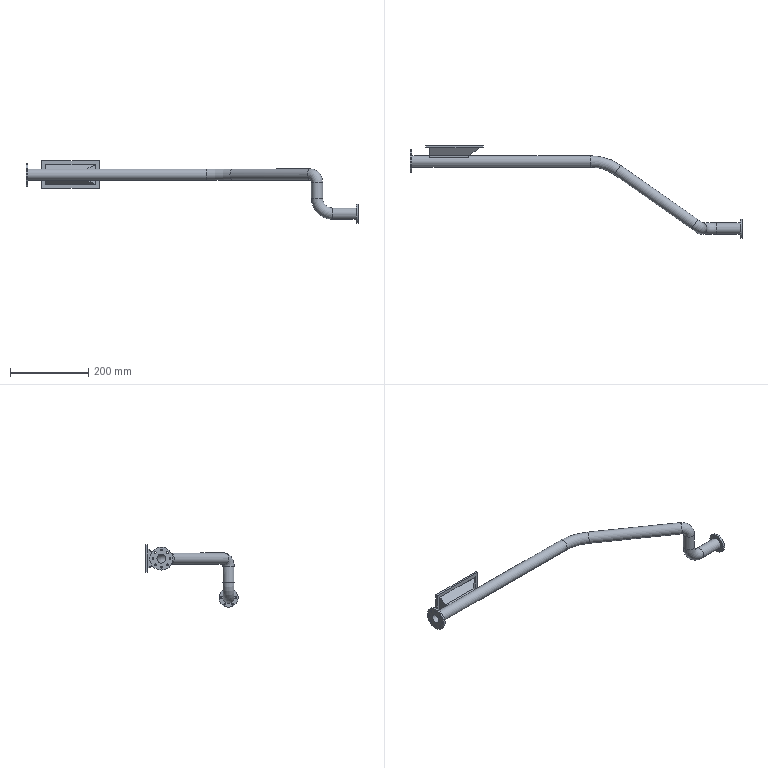Part | STEP file | Pipe Coal Feder | 1 solid | 58 faces | box 850.746 x 236.073 x 160 mm | volume 290347 mm3 | plane 28 | cylinder 24 | torus 6 | commonest cylinder face diameters 4.134 x14 23 x4 29 x4 49 x1 59 x1